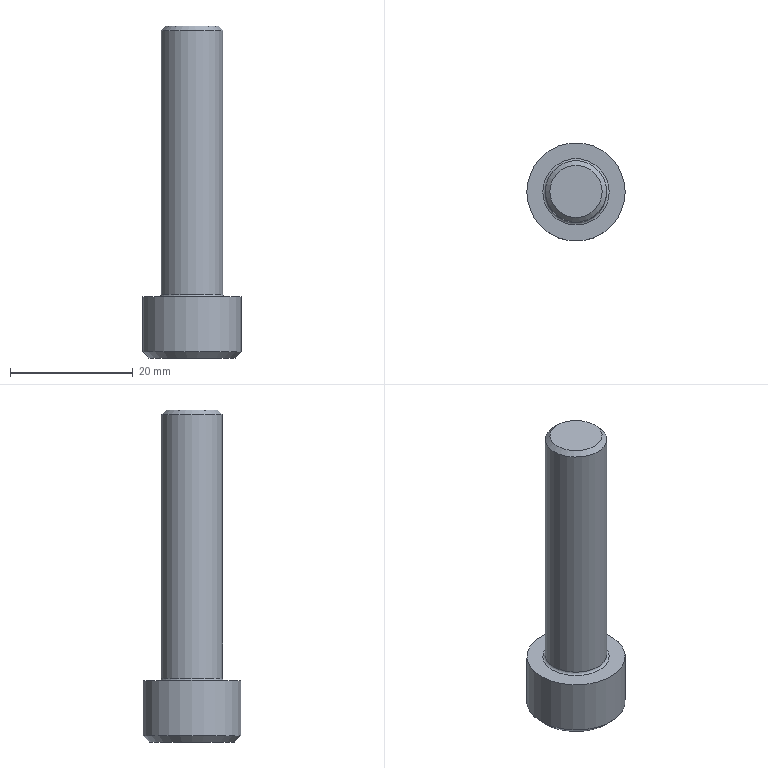Part | STEP file | solid 119 | 1 solid | 21 faces | box 16 x 16 x 54 mm | volume 5157 mm3 | plane 10 | sphere 6 | cylinder 2 | cone 2 | torus 1 | commonest cylinder face diameters 10 x1 16 x1